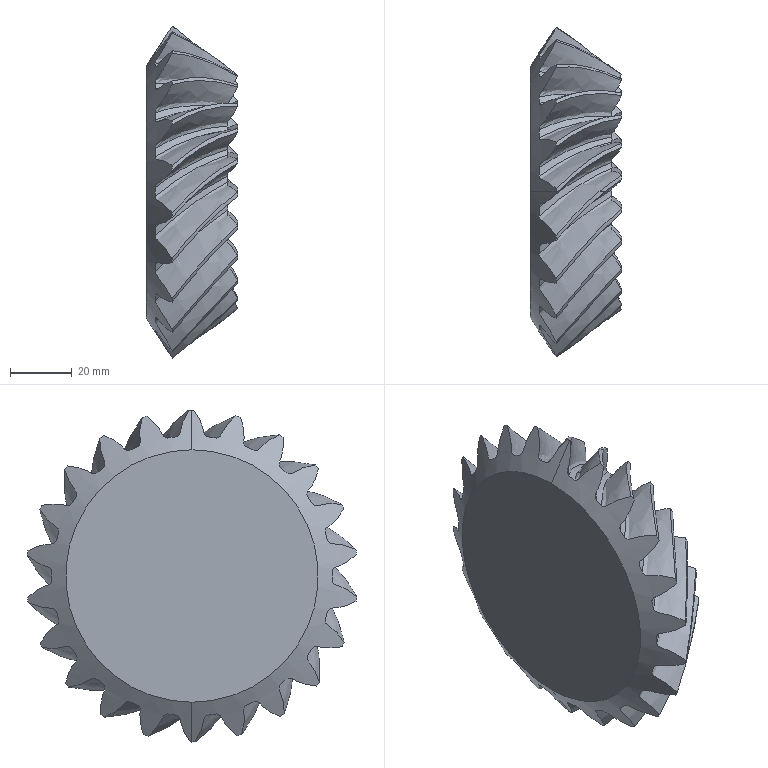Part | NX | features BREP 1 | 1 solid | 116 faces | box 29.455 x 106.309 x 107.135 mm | volume 151425 mm3 | spline 66 | cone 48 | plane 2